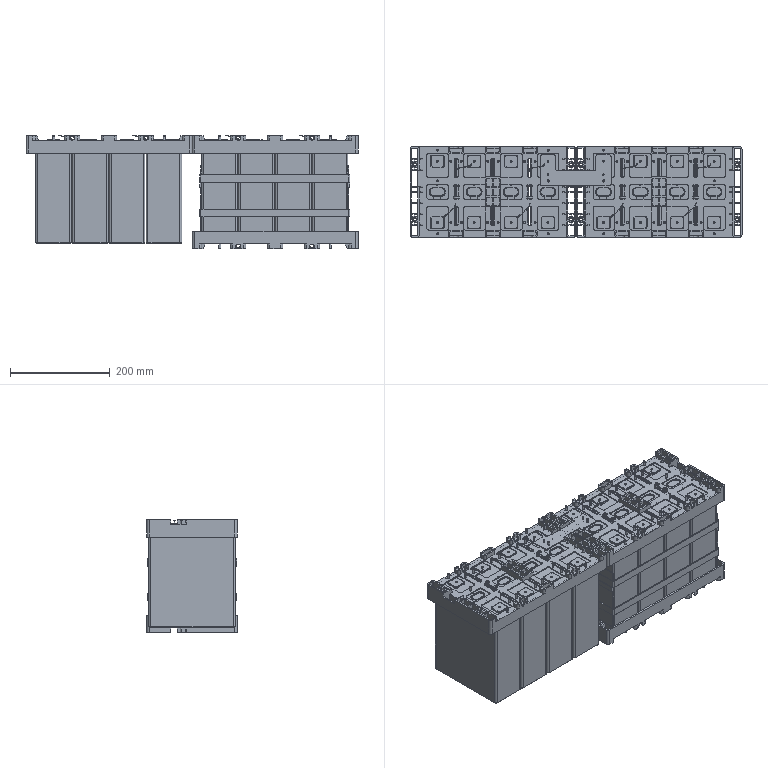Part | NX | features BREP 27 | 27 solids | 4564 faces | volume 21203019 mm3 | plane 2954 | cylinder 1358 | cone 192 | spline 48 | torus 12 | commonest cylinder face diameters 6 x364 4 x348 10 x146 2 x96 8 x68 4.22 x48